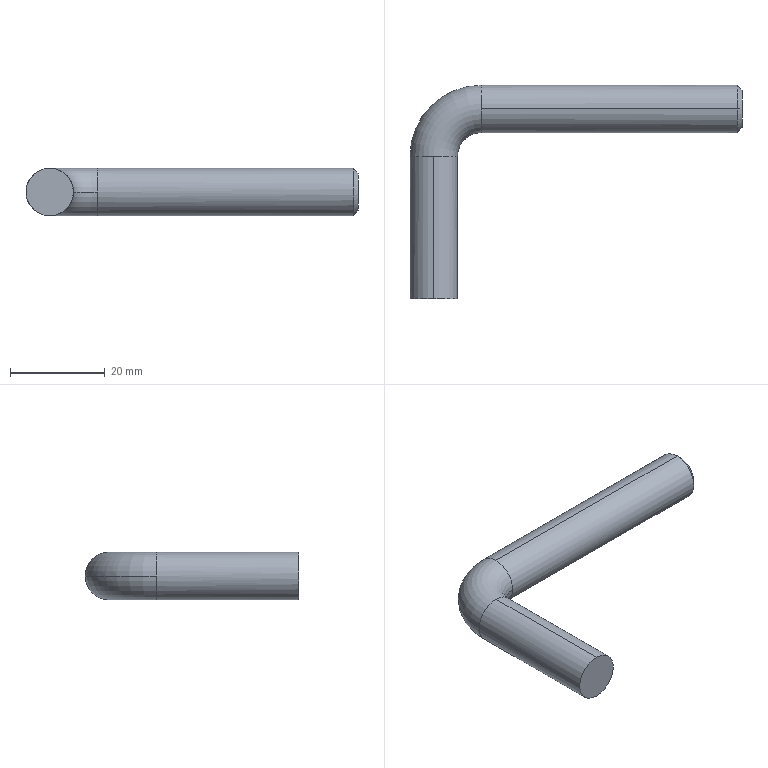Part | SolidWorks | features BaseBody 1 | 1 solid | 10 faces | box 70 x 45 x 10 mm | volume 7895 mm3 | cylinder 4 | cone 2 | plane 2 | torus 2 | commonest cylinder face diameters 10 x4
STEP:
#1=CARTESIAN_POINT('',(65.,40.,-4.));
#2=VERTEX_POINT('',#1);
#3=CARTESIAN_POINT('',(64.,40.,-5.));
#4=VERTEX_POINT('',#3);
#5=CARTESIAN_POINT('',(65.,40.,-4.));
#6=DIRECTION('',(-0.7071,0.,-0.7071));
#7=VECTOR('',#6,1000.);
#8=LINE('',#5,#7);
#9=EDGE_CURVE('',#2,#4,#8,.T.);
#10=ORIENTED_EDGE('',*,*,#9,.F.);
#11=CARTESIAN_POINT('',(65.,40.,4.));
#12=VERTEX_POINT('',#11);
#13=CARTESIAN_POINT('',(65.,40.,0.));
#14=DIRECTION('',(1.,0.,0.));
#15=DIRECTION('',(0.,0.,-1.));
#16=AXIS2_PLACEMENT_3D('',#13,#14,#15);
#17=CIRCLE('',#16,4.);
#18=EDGE_CURVE('',#12,#2,#17,.T.);
#19=ORIENTED_EDGE('',*,*,#18,.F.);
#20=CARTESIAN_POINT('',(64.,40.,5.));
#21=VERTEX_POINT('',#20);
#22=CARTESIAN_POINT('',(65.,40.,4.));
#23=DIRECTION('',(-0.7071,0.,0.7071));
#24=VECTOR('',#23,1000.);
#25=LINE('',#22,#24);
#26=EDGE_CURVE('',#12,#21,#25,.T.);
#27=ORIENTED_EDGE('',*,*,#26,.T.);
#28=CARTESIAN_POINT('',(64.,40.,0.));
#29=DIRECTION('',(-1.,0.,0.));
#30=DIRECTION('',(0.,0.,-1.));
#31=AXIS2_PLACEMENT_3D('',#28,#29,#30);
#32=CIRCLE('',#31,5.);
#33=EDGE_CURVE('',#4,#21,#32,.T.);
#34=ORIENTED_EDGE('',*,*,#33,.F.);
#35=EDGE_LOOP('',(#10,#19,#27,#34));
#36=FACE_OUTER_BOUND('',#35,.T.);
#37=CARTESIAN_POINT('',(65.,40.,0.));
#38=DIRECTION('',(-1.,0.,0.));
#39=DIRECTION('',(0.,0.,1.));
#40=AXIS2_PLACEMENT_3D('',#37,#38,#39);
#41=CONICAL_SURFACE('',#40,4.,0.7854);
#42=ADVANCED_FACE('',(#36),#41,.T.);
#43=CARTESIAN_POINT('',(0.,0.,5.));
#44=VERTEX_POINT('',#43);
#45=CARTESIAN_POINT('',(0.,0.,-5.));
#46=VERTEX_POINT('',#45);
#47=CARTESIAN_POINT('',(0.,0.,0.));
#48=DIRECTION('',(0.,1.,0.));
#49=DIRECTION('',(0.,0.,1.));
#50=AXIS2_PLACEMENT_3D('',#47,#48,#49);
#51=CIRCLE('',#50,5.);
#52=EDGE_CURVE('',#44,#46,#51,.T.);
#53=ORIENTED_EDGE('',*,*,#52,.F.);
#54=CARTESIAN_POINT('',(0.,0.,0.));
#55=DIRECTION('',(0.,1.,0.));
#56=DIRECTION('',(0.,0.,1.));
#57=AXIS2_PLACEMENT_3D('',#54,#55,#56);
#58=CIRCLE('',#57,5.);
#59=EDGE_CURVE('',#46,#44,#58,.T.);
#60=ORIENTED_EDGE('',*,*,#59,.F.);
#61=EDGE_LOOP('',(#53,#60));
#62=FACE_OUTER_BOUND('',#61,.T.);
#63=CARTESIAN_POINT('',(0.,0.,0.));
#64=DIRECTION('',(0.,1.,0.));
#65=DIRECTION('',(1.,0.,0.));
#66=AXIS2_PLACEMENT_3D('',#63,#64,#65);
#67=PLANE('',#66);
#68=ADVANCED_FACE('',(#62),#67,.F.);
#69=ORIENTED_EDGE('',*,*,#18,.T.);
#70=CARTESIAN_POINT('',(65.,40.,0.));
#71=DIRECTION('',(1.,0.,0.));
#72=DIRECTION('',(0.,0.,-1.));
#73=AXIS2_PLACEMENT_3D('',#70,#71,#72);
#74=CIRCLE('',#73,4.);
#75=EDGE_CURVE('',#2,#12,#74,.T.);
#76=ORIENTED_EDGE('',*,*,#75,.T.);
#77=EDGE_LOOP('',(#69,#76));
#78=FACE_OUTER_BOUND('',#77,.T.);
#79=CARTESIAN_POINT('',(65.,40.,0.));
#80=DIRECTION('',(1.,0.,0.));
#81=DIRECTION('',(0.,1.,0.));
#82=AXIS2_PLACEMENT_3D('',#79,#80,#81);
#83=PLANE('',#82);
#84=ADVANCED_FACE('',(#78),#83,.T.);
#85=CARTESIAN_POINT('',(0.,30.,-5.));
#86=VERTEX_POINT('',#85);
#87=CARTESIAN_POINT('',(0.,0.,-5.));
#88=DIRECTION('',(0.,1.,0.));
#89=VECTOR('',#88,1000.);
#90=LINE('',#87,#89);
#91=EDGE_CURVE('',#46,#86,#90,.T.);
#92=ORIENTED_EDGE('',*,*,#91,.F.);
#93=ORIENTED_EDGE('',*,*,#59,.T.);
#94=CARTESIAN_POINT('',(0.,30.,5.));
#95=VERTEX_POINT('',#94);
#96=CARTESIAN_POINT('',(0.,0.,5.));
#97=DIRECTION('',(0.,1.,0.));
#98=VECTOR('',#97,1000.);
#99=LINE('',#96,#98);
#100=EDGE_CURVE('',#44,#95,#99,.T.);
#101=ORIENTED_EDGE('',*,*,#100,.T.);
#102=CARTESIAN_POINT('',(-5.,30.,0.));
#103=VERTEX_POINT('',#102);
#104=CARTESIAN_POINT('',(0.,30.,0.));
#105=DIRECTION('',(0.,1.,0.));
#106=DIRECTION('',(0.,0.,1.));
#107=AXIS2_PLACEMENT_3D('',#104,#105,#106);
#108=CIRCLE('',#107,5.);
#109=EDGE_CURVE('',#103,#95,#108,.T.);
#110=ORIENTED_EDGE('',*,*,#109,.F.);
#111=CARTESIAN_POINT('',(0.,30.,0.));
#112=DIRECTION('',(0.,1.,0.));
#113=DIRECTION('',(0.,0.,1.));
#114=AXIS2_PLACEMENT_3D('',#111,#112,#113);
#115=CIRCLE('',#114,5.);
#116=EDGE_CURVE('',#86,#103,#115,.T.);
#117=ORIENTED_EDGE('',*,*,#116,.F.);
#118=EDGE_LOOP('',(#92,#93,#101,#110,#117));
#119=FACE_OUTER_BOUND('',#118,.T.);
#120=CARTESIAN_POINT('',(0.,0.,0.));
#121=DIRECTION('',(0.,1.,0.));
#122=DIRECTION('',(0.,0.,1.));
#123=AXIS2_PLACEMENT_3D('',#120,#121,#122);
#124=CYLINDRICAL_SURFACE('',#123,5.);
#125=ADVANCED_FACE('',(#119),#124,.T.);
#126=CARTESIAN_POINT('',(10.,45.,0.));
#127=VERTEX_POINT('',#126);
#128=CARTESIAN_POINT('',(10.,30.,0.));
#129=DIRECTION('',(0.,0.,-1.));
#130=DIRECTION('',(-1.,0.,0.));
#131=AXIS2_PLACEMENT_3D('',#128,#129,#130);
#132=CIRCLE('',#131,15.);
#133=EDGE_CURVE('',#103,#127,#132,.T.);
#134=ORIENTED_EDGE('',*,*,#133,.F.);
#135=ORIENTED_EDGE('',*,*,#109,.T.);
#136=CARTESIAN_POINT('',(5.,30.,0.));
#137=VERTEX_POINT('',#136);
#138=CARTESIAN_POINT('',(0.,30.,0.));
#139=DIRECTION('',(0.,1.,0.));
#140=DIRECTION('',(0.,0.,1.));
#141=AXIS2_PLACEMENT_3D('',#138,#139,#140);
#142=CIRCLE('',#141,5.);
#143=EDGE_CURVE('',#95,#137,#142,.T.);
#144=ORIENTED_EDGE('',*,*,#143,.T.);
#145=CARTESIAN_POINT('',(10.,35.,0.));
#146=VERTEX_POINT('',#145);
#147=CARTESIAN_POINT('',(10.,30.,0.));
#148=DIRECTION('',(0.,0.,-1.));
#149=DIRECTION('',(-1.,0.,0.));
#150=AXIS2_PLACEMENT_3D('',#147,#148,#149);
#151=CIRCLE('',#150,5.);
#152=EDGE_CURVE('',#137,#146,#151,.T.);
#153=ORIENTED_EDGE('',*,*,#152,.T.);
#154=CARTESIAN_POINT('',(10.,40.,5.));
#155=VERTEX_POINT('',#154);
#156=CARTESIAN_POINT('',(10.,40.,0.));
#157=DIRECTION('',(1.,0.,0.));
#158=DIRECTION('',(0.,0.,1.));
#159=AXIS2_PLACEMENT_3D('',#156,#157,#158);
#160=CIRCLE('',#159,5.);
#161=EDGE_CURVE('',#155,#146,#160,.T.);
#162=ORIENTED_EDGE('',*,*,#161,.F.);
#163=CARTESIAN_POINT('',(10.,40.,0.));
#164=DIRECTION('',(1.,0.,0.));
#165=DIRECTION('',(0.,0.,1.));
#166=AXIS2_PLACEMENT_3D('',#163,#164,#165);
#167=CIRCLE('',#166,5.);
#168=EDGE_CURVE('',#127,#155,#167,.T.);
#169=ORIENTED_EDGE('',*,*,#168,.F.);
#170=EDGE_LOOP('',(#134,#135,#144,#153,#162,#169));
#171=FACE_OUTER_BOUND('',#170,.T.);
#172=CARTESIAN_POINT('',(10.,30.,0.));
#173=DIRECTION('',(0.,0.,-1.));
#174=DIRECTION('',(-1.,0.,0.));
#175=AXIS2_PLACEMENT_3D('',#172,#173,#174);
#176=TOROIDAL_SURFACE('',#175,10.,5.);
#177=ADVANCED_FACE('',(#171),#176,.T.);
#178=CARTESIAN_POINT('',(10.,40.,5.));
#179=DIRECTION('',(1.,0.,0.));
#180=VECTOR('',#179,1000.);
#181=LINE('',#178,#180);
#182=EDGE_CURVE('',#155,#21,#181,.T.);
#183=ORIENTED_EDGE('',*,*,#182,.F.);
#184=ORIENTED_EDGE('',*,*,#161,.T.);
#185=CARTESIAN_POINT('',(10.,40.,-5.));
#186=VERTEX_POINT('',#185);
#187=CARTESIAN_POINT('',(10.,40.,0.));
#188=DIRECTION('',(1.,0.,0.));
#189=DIRECTION('',(0.,0.,1.));
#190=AXIS2_PLACEMENT_3D('',#187,#188,#189);
#191=CIRCLE('',#190,5.);
#192=EDGE_CURVE('',#146,#186,#191,.T.);
#193=ORIENTED_EDGE('',*,*,#192,.T.);
#194=CARTESIAN_POINT('',(10.,40.,-5.));
#195=DIRECTION('',(1.,0.,0.));
#196=VECTOR('',#195,1000.);
#197=LINE('',#194,#196);
#198=EDGE_CURVE('',#186,#4,#197,.T.);
#199=ORIENTED_EDGE('',*,*,#198,.T.);
#200=ORIENTED_EDGE('',*,*,#33,.T.);
#201=EDGE_LOOP('',(#183,#184,#193,#199,#200));
#202=FACE_OUTER_BOUND('',#201,.T.);
#203=CARTESIAN_POINT('',(10.,40.,0.));
#204=DIRECTION('',(1.,0.,0.));
#205=DIRECTION('',(0.,0.,-1.));
#206=AXIS2_PLACEMENT_3D('',#203,#204,#205);
#207=CYLINDRICAL_SURFACE('',#206,5.);
#208=ADVANCED_FACE('',(#202),#207,.T.);
#209=ORIENTED_EDGE('',*,*,#52,.T.);
#210=ORIENTED_EDGE('',*,*,#91,.T.);
#211=CARTESIAN_POINT('',(0.,30.,0.));
#212=DIRECTION('',(0.,1.,0.));
#213=DIRECTION('',(0.,0.,1.));
#214=AXIS2_PLACEMENT_3D('',#211,#212,#213);
#215=CIRCLE('',#214,5.);
#216=EDGE_CURVE('',#137,#86,#215,.T.);
#217=ORIENTED_EDGE('',*,*,#216,.F.);
#218=ORIENTED_EDGE('',*,*,#143,.F.);
#219=ORIENTED_EDGE('',*,*,#100,.F.);
#220=EDGE_LOOP('',(#209,#210,#217,#218,#219));
#221=FACE_OUTER_BOUND('',#220,.T.);
#222=CARTESIAN_POINT('',(0.,0.,0.));
#223=DIRECTION('',(0.,1.,0.));
#224=DIRECTION('',(0.,0.,1.));
#225=AXIS2_PLACEMENT_3D('',#222,#223,#224);
#226=CYLINDRICAL_SURFACE('',#225,5.);
#227=ADVANCED_FACE('',(#221),#226,.T.);
#228=CARTESIAN_POINT('',(10.,40.,0.));
#229=DIRECTION('',(1.,0.,0.));
#230=DIRECTION('',(0.,0.,1.));
#231=AXIS2_PLACEMENT_3D('',#228,#229,#230);
#232=CIRCLE('',#231,5.);
#233=EDGE_CURVE('',#186,#127,#232,.T.);
#234=ORIENTED_EDGE('',*,*,#233,.T.);
#235=ORIENTED_EDGE('',*,*,#168,.T.);
#236=ORIENTED_EDGE('',*,*,#182,.T.);
#237=CARTESIAN_POINT('',(64.,40.,0.));
#238=DIRECTION('',(-1.,0.,0.));
#239=DIRECTION('',(0.,0.,-1.));
#240=AXIS2_PLACEMENT_3D('',#237,#238,#239);
#241=CIRCLE('',#240,5.);
#242=EDGE_CURVE('',#21,#4,#241,.T.);
#243=ORIENTED_EDGE('',*,*,#242,.T.);
#244=ORIENTED_EDGE('',*,*,#198,.F.);
#245=EDGE_LOOP('',(#234,#235,#236,#243,#244));
#246=FACE_OUTER_BOUND('',#245,.T.);
#247=CARTESIAN_POINT('',(10.,40.,0.));
#248=DIRECTION('',(1.,0.,0.));
#249=DIRECTION('',(0.,0.,-1.));
#250=AXIS2_PLACEMENT_3D('',#247,#248,#249);
#251=CYLINDRICAL_SURFACE('',#250,5.);
#252=ADVANCED_FACE('',(#246),#251,.T.);
#253=ORIENTED_EDGE('',*,*,#75,.F.);
#254=ORIENTED_EDGE('',*,*,#9,.T.);
#255=ORIENTED_EDGE('',*,*,#242,.F.);
#256=ORIENTED_EDGE('',*,*,#26,.F.);
#257=EDGE_LOOP('',(#253,#254,#255,#256));
#258=FACE_OUTER_BOUND('',#257,.T.);
#259=CARTESIAN_POINT('',(65.,40.,0.));
#260=DIRECTION('',(-1.,0.,0.));
#261=DIRECTION('',(0.,0.,1.));
#262=AXIS2_PLACEMENT_3D('',#259,#260,#261);
#263=CONICAL_SURFACE('',#262,4.,0.7854);
#264=ADVANCED_FACE('',(#258),#263,.T.);
#265=ORIENTED_EDGE('',*,*,#116,.T.);
#266=ORIENTED_EDGE('',*,*,#133,.T.);
#267=ORIENTED_EDGE('',*,*,#233,.F.);
#268=ORIENTED_EDGE('',*,*,#192,.F.);
#269=ORIENTED_EDGE('',*,*,#152,.F.);
#270=ORIENTED_EDGE('',*,*,#216,.T.);
#271=EDGE_LOOP('',(#265,#266,#267,#268,#269,#270));
#272=FACE_OUTER_BOUND('',#271,.T.);
#273=CARTESIAN_POINT('',(10.,30.,0.));
#274=DIRECTION('',(0.,0.,-1.));
#275=DIRECTION('',(-1.,0.,0.));
#276=AXIS2_PLACEMENT_3D('',#273,#274,#275);
#277=TOROIDAL_SURFACE('',#276,10.,5.);
#278=ADVANCED_FACE('',(#272),#277,.T.);
#279=CLOSED_SHELL('',(#42,#68,#84,#125,#177,#208,#227,#252,#264,#278));
#280=MANIFOLD_SOLID_BREP('',#279);
#281=CARTESIAN_POINT('',(0.,0.,0.));
#282=DIRECTION('',(0.,0.,1.));
#283=DIRECTION('',(1.,0.,0.));
#284=AXIS2_PLACEMENT_3D('',#281,#282,#283);
#285=(LENGTH_UNIT()NAMED_UNIT(*)SI_UNIT(.MILLI.,.METRE.));
#286=UNCERTAINTY_MEASURE_WITH_UNIT(LENGTH_MEASURE(0.00001),#285,'','');
#287=(NAMED_UNIT(*)PLANE_ANGLE_UNIT()SI_UNIT($,.RADIAN.));
#288=(NAMED_UNIT(*)SI_UNIT($,.STERADIAN.)SOLID_ANGLE_UNIT());
#289=(GEOMETRIC_REPRESENTATION_CONTEXT(3)GLOBAL_UNCERTAINTY_ASSIGNED_CONTEXT((#286))GLOBAL_UNIT_ASSIGNED_CONTEXT((#285,#287,#288))REPRESENTATION_CONTEXT('',''));
#290=ADVANCED_BREP_SHAPE_REPRESENTATION('',(#280,#284),#289);